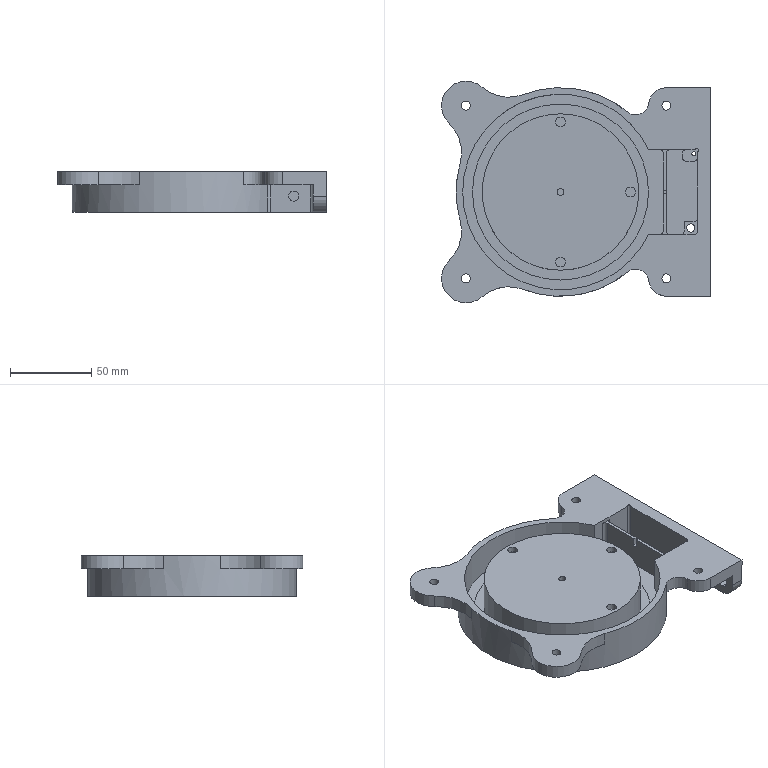NC program | NX | posted with a generic post | part box 165 x 136 x 25 mm
Lines 1 to 70 of 16615:
N10 G17 G21 G94 G90
(FLOOR_WALL , TOOL : D63)
N12 T01 M6
N14 G54
N16 G17 G0 G90 X122. Y-72.997 S6500 M3
N18 G43 Z30. H1
N20 Z3.
N22 G94 G1 Z0. F1250.
N24 X119.
N26 X-119.
N28 Y-61.839
N30 Y-32.731
N32 X119.
N34 Y7.534
N36 X-119.
N38 Y47.8
N40 X119.
N42 X122.
N44 Z3.
N46 G0 Z30.
N48 M5
(DRILLING , TOOL : D6A45)
N50 T07 M6
N52 G54
N54 G17 G0 G90 X67.5 Y-53. S5000 M3
N56 G43 Z30. H7
N58 G94 G81 G98 Z-1. F250. R3.
N60 X9.5 Y-43.
N62 Y0.
N64 X-33.5
N66 X-55.5 Y-53.
N68 X-74.146 Y-25.646
N70 X-55.5 Y53.
N72 X9.5 Y43.
N74 X67.5 Y53.
N76 G80
N78 G0 X67.5 Y53. Z30.
N80 M5
(DRILLING_COPY , TOOL : 4.2ZT)
N82 T14 M6
N84 G54
N86 G17 G0 G90 X67.5 Y53. S2000 M3
N88 G43 Z30. H14
N90 G94 G83 G98 Z-10.762 F250. Q2. R3.
N92 Y-53.
N94 X9.5 Y0. Z-10.
N96 X-55.5 Y-53. Z-10.762
N98 Y53.
N100 G80
N102 G0 X-55.5 Y53. Z30.
N104 M5
(DRILLING_COPY_COPY_1 , TOOL : 2.0ZT)
N106 T12 M6
N108 G54
N110 G17 G0 G90 X-74.146 Y-25.646 S2000 M3
N112 G43 Z30. H12
N114 G94 G83 G98 Z-24.101 F120. Q2. R3.
N116 G80
N118 G0 X-74.146 Y-25.646 Z30.
N120 M5